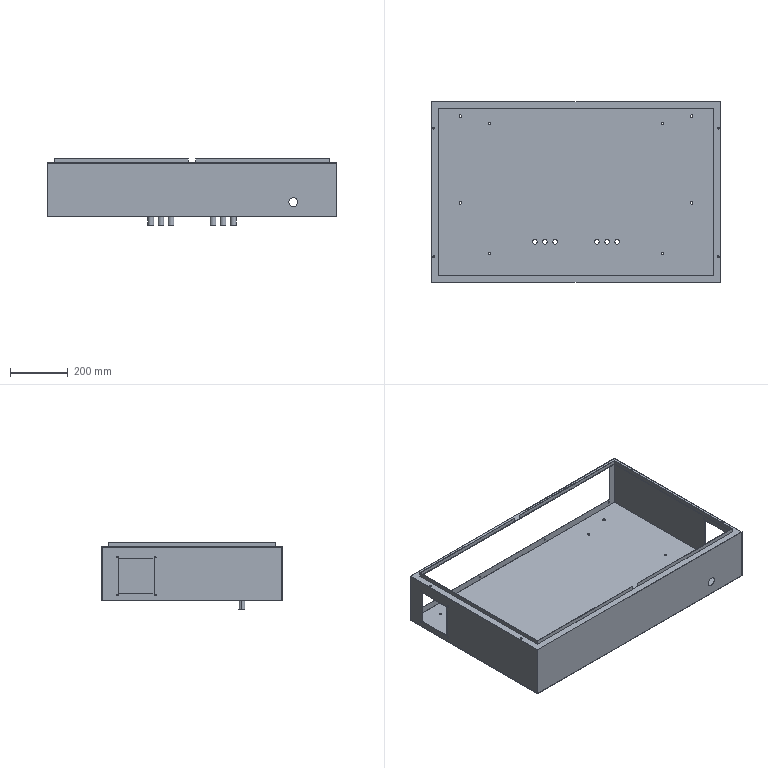Part | STEP file | 1 solid | 128 faces | box 1000 x 625 x 230.5 mm | volume 1788128 mm3 | cylinder 82 | plane 46 | commonest cylinder face diameters 4.2 x16 5 x16 16 x12 20 x12 6.5 x8 8.5 x8